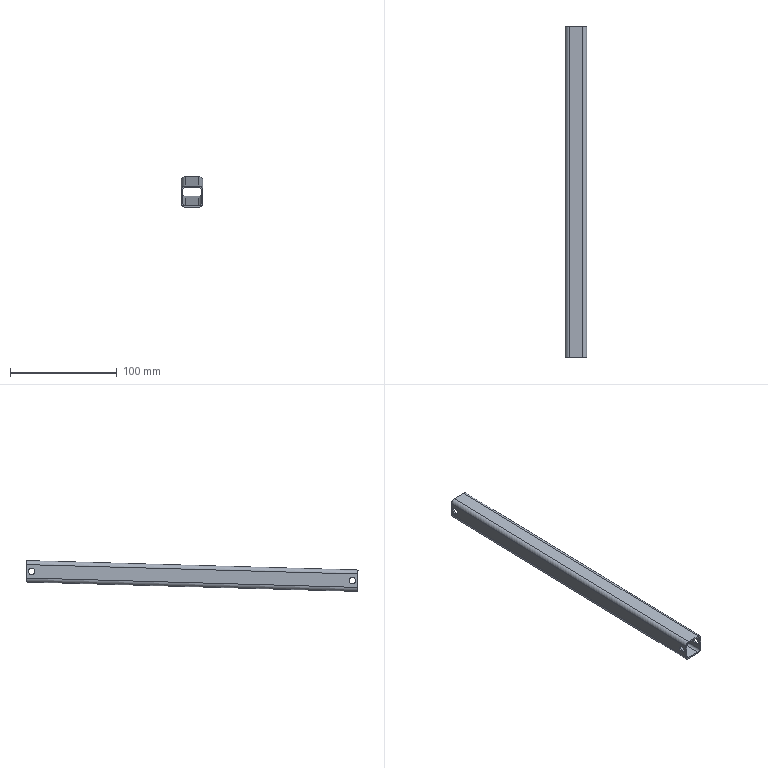Part | SolidWorks | features BaseBody 1 | 1 solid | 26 faces | box 20 x 310.443 x 28.789 mm | volume 31845 mm3 | cylinder 16 | plane 10 | commonest cylinder face diameters 6 x8 4.5 x4 7.5 x4
STEP:
#1=CARTESIAN_POINT('',(-3.273,-26.055,-774.101));
#2=VERTEX_POINT('',#1);
#3=CARTESIAN_POINT('',(-3.273,-32.052,-774.271));
#4=VERTEX_POINT('',#3);
#5=CARTESIAN_POINT('',(-3.273,-29.054,-774.186));
#6=DIRECTION('',(1.,0.,0.));
#7=DIRECTION('',(0.,-0.9996,-0.02838));
#8=AXIS2_PLACEMENT_3D('',#5,#6,#7);
#9=CIRCLE('',#8,3.);
#10=EDGE_CURVE('',#2,#4,#9,.T.);
#11=ORIENTED_EDGE('',*,*,#10,.F.);
#12=CARTESIAN_POINT('',(-1.773,-26.055,-774.101));
#13=VERTEX_POINT('',#12);
#14=CARTESIAN_POINT('',(-21.773,-26.055,-774.101));
#15=DIRECTION('',(1.,0.,0.));
#16=VECTOR('',#15,1000.);
#17=LINE('',#14,#16);
#18=EDGE_CURVE('',#2,#13,#17,.T.);
#19=ORIENTED_EDGE('',*,*,#18,.T.);
#20=CARTESIAN_POINT('',(-1.773,-32.052,-774.271));
#21=VERTEX_POINT('',#20);
#22=CARTESIAN_POINT('',(-1.773,-29.054,-774.186));
#23=DIRECTION('',(-1.,0.,0.));
#24=DIRECTION('',(0.,-0.9996,-0.02838));
#25=AXIS2_PLACEMENT_3D('',#22,#23,#24);
#26=CIRCLE('',#25,3.);
#27=EDGE_CURVE('',#21,#13,#26,.T.);
#28=ORIENTED_EDGE('',*,*,#27,.F.);
#29=CARTESIAN_POINT('',(-21.773,-32.052,-774.271));
#30=DIRECTION('',(1.,0.,0.));
#31=VECTOR('',#30,1000.);
#32=LINE('',#29,#31);
#33=EDGE_CURVE('',#4,#21,#32,.T.);
#34=ORIENTED_EDGE('',*,*,#33,.F.);
#35=EDGE_LOOP('',(#11,#19,#28,#34));
#36=FACE_OUTER_BOUND('',#35,.T.);
#37=CARTESIAN_POINT('',(-21.773,-29.054,-774.186));
#38=DIRECTION('',(1.,0.,0.));
#39=DIRECTION('',(0.,-0.9996,-0.02838));
#40=AXIS2_PLACEMENT_3D('',#37,#38,#39);
#41=CYLINDRICAL_SURFACE('',#40,3.);
#42=ADVANCED_FACE('',(#36),#41,.F.);
#43=CARTESIAN_POINT('',(-21.773,-26.055,-774.101));
#44=VERTEX_POINT('',#43);
#45=CARTESIAN_POINT('',(-21.773,-32.052,-774.271));
#46=VERTEX_POINT('',#45);
#47=CARTESIAN_POINT('',(-21.773,-29.054,-774.186));
#48=DIRECTION('',(1.,0.,0.));
#49=DIRECTION('',(0.,-0.9996,-0.02838));
#50=AXIS2_PLACEMENT_3D('',#47,#48,#49);
#51=CIRCLE('',#50,3.);
#52=EDGE_CURVE('',#44,#46,#51,.T.);
#53=ORIENTED_EDGE('',*,*,#52,.F.);
#54=CARTESIAN_POINT('',(-20.273,-26.055,-774.101));
#55=VERTEX_POINT('',#54);
#56=CARTESIAN_POINT('',(-21.773,-26.055,-774.101));
#57=DIRECTION('',(1.,0.,0.));
#58=VECTOR('',#57,1000.);
#59=LINE('',#56,#58);
#60=EDGE_CURVE('',#44,#55,#59,.T.);
#61=ORIENTED_EDGE('',*,*,#60,.T.);
#62=CARTESIAN_POINT('',(-20.273,-32.052,-774.271));
#63=VERTEX_POINT('',#62);
#64=CARTESIAN_POINT('',(-20.273,-29.054,-774.186));
#65=DIRECTION('',(-1.,0.,0.));
#66=DIRECTION('',(0.,-0.9996,-0.02838));
#67=AXIS2_PLACEMENT_3D('',#64,#65,#66);
#68=CIRCLE('',#67,3.);
#69=EDGE_CURVE('',#63,#55,#68,.T.);
#70=ORIENTED_EDGE('',*,*,#69,.F.);
#71=CARTESIAN_POINT('',(-21.773,-32.052,-774.271));
#72=DIRECTION('',(1.,0.,0.));
#73=VECTOR('',#72,1000.);
#74=LINE('',#71,#73);
#75=EDGE_CURVE('',#46,#63,#74,.T.);
#76=ORIENTED_EDGE('',*,*,#75,.F.);
#77=EDGE_LOOP('',(#53,#61,#70,#76));
#78=FACE_OUTER_BOUND('',#77,.T.);
#79=CARTESIAN_POINT('',(-21.773,-29.054,-774.186));
#80=DIRECTION('',(1.,0.,0.));
#81=DIRECTION('',(0.,-0.9996,-0.02838));
#82=AXIS2_PLACEMENT_3D('',#79,#80,#81);
#83=CYLINDRICAL_SURFACE('',#82,3.);
#84=ADVANCED_FACE('',(#78),#83,.F.);
#85=CARTESIAN_POINT('',(-3.273,273.824,-765.587));
#86=VERTEX_POINT('',#85);
#87=CARTESIAN_POINT('',(-3.273,267.827,-765.757));
#88=VERTEX_POINT('',#87);
#89=CARTESIAN_POINT('',(-3.273,270.826,-765.672));
#90=DIRECTION('',(1.,0.,0.));
#91=DIRECTION('',(0.,-0.9996,-0.02838));
#92=AXIS2_PLACEMENT_3D('',#89,#90,#91);
#93=CIRCLE('',#92,3.);
#94=EDGE_CURVE('',#86,#88,#93,.T.);
#95=ORIENTED_EDGE('',*,*,#94,.F.);
#96=CARTESIAN_POINT('',(-1.773,273.824,-765.587));
#97=VERTEX_POINT('',#96);
#98=CARTESIAN_POINT('',(-21.773,273.824,-765.587));
#99=DIRECTION('',(1.,0.,0.));
#100=VECTOR('',#99,1000.);
#101=LINE('',#98,#100);
#102=EDGE_CURVE('',#86,#97,#101,.T.);
#103=ORIENTED_EDGE('',*,*,#102,.T.);
#104=CARTESIAN_POINT('',(-1.773,267.827,-765.757));
#105=VERTEX_POINT('',#104);
#106=CARTESIAN_POINT('',(-1.773,270.826,-765.672));
#107=DIRECTION('',(-1.,0.,0.));
#108=DIRECTION('',(0.,-0.9996,-0.02838));
#109=AXIS2_PLACEMENT_3D('',#106,#107,#108);
#110=CIRCLE('',#109,3.);
#111=EDGE_CURVE('',#105,#97,#110,.T.);
#112=ORIENTED_EDGE('',*,*,#111,.F.);
#113=CARTESIAN_POINT('',(-21.773,267.827,-765.757));
#114=DIRECTION('',(1.,0.,0.));
#115=VECTOR('',#114,1000.);
#116=LINE('',#113,#115);
#117=EDGE_CURVE('',#88,#105,#116,.T.);
#118=ORIENTED_EDGE('',*,*,#117,.F.);
#119=EDGE_LOOP('',(#95,#103,#112,#118));
#120=FACE_OUTER_BOUND('',#119,.T.);
#121=CARTESIAN_POINT('',(-21.773,270.826,-765.672));
#122=DIRECTION('',(1.,0.,0.));
#123=DIRECTION('',(0.,-0.9996,-0.02838));
#124=AXIS2_PLACEMENT_3D('',#121,#122,#123);
#125=CYLINDRICAL_SURFACE('',#124,3.);
#126=ADVANCED_FACE('',(#120),#125,.F.);
#127=CARTESIAN_POINT('',(-21.773,273.824,-765.587));
#128=VERTEX_POINT('',#127);
#129=CARTESIAN_POINT('',(-21.773,267.827,-765.757));
#130=VERTEX_POINT('',#129);
#131=CARTESIAN_POINT('',(-21.773,270.826,-765.672));
#132=DIRECTION('',(1.,0.,0.));
#133=DIRECTION('',(0.,-0.9996,-0.02838));
#134=AXIS2_PLACEMENT_3D('',#131,#132,#133);
#135=CIRCLE('',#134,3.);
#136=EDGE_CURVE('',#128,#130,#135,.T.);
#137=ORIENTED_EDGE('',*,*,#136,.F.);
#138=CARTESIAN_POINT('',(-20.273,273.824,-765.587));
#139=VERTEX_POINT('',#138);
#140=CARTESIAN_POINT('',(-21.773,273.824,-765.587));
#141=DIRECTION('',(1.,0.,0.));
#142=VECTOR('',#141,1000.);
#143=LINE('',#140,#142);
#144=EDGE_CURVE('',#128,#139,#143,.T.);
#145=ORIENTED_EDGE('',*,*,#144,.T.);
#146=CARTESIAN_POINT('',(-20.273,267.827,-765.757));
#147=VERTEX_POINT('',#146);
#148=CARTESIAN_POINT('',(-20.273,270.826,-765.672));
#149=DIRECTION('',(-1.,0.,0.));
#150=DIRECTION('',(0.,-0.9996,-0.02838));
#151=AXIS2_PLACEMENT_3D('',#148,#149,#150);
#152=CIRCLE('',#151,3.);
#153=EDGE_CURVE('',#147,#139,#152,.T.);
#154=ORIENTED_EDGE('',*,*,#153,.F.);
#155=CARTESIAN_POINT('',(-21.773,267.827,-765.757));
#156=DIRECTION('',(1.,0.,0.));
#157=VECTOR('',#156,1000.);
#158=LINE('',#155,#157);
#159=EDGE_CURVE('',#130,#147,#158,.T.);
#160=ORIENTED_EDGE('',*,*,#159,.F.);
#161=EDGE_LOOP('',(#137,#145,#154,#160));
#162=FACE_OUTER_BOUND('',#161,.T.);
#163=CARTESIAN_POINT('',(-21.773,270.826,-765.672));
#164=DIRECTION('',(1.,0.,0.));
#165=DIRECTION('',(0.,-0.9996,-0.02838));
#166=AXIS2_PLACEMENT_3D('',#163,#164,#165);
#167=CYLINDRICAL_SURFACE('',#166,3.);
#168=ADVANCED_FACE('',(#162),#167,.F.);
#169=CARTESIAN_POINT('',(-18.023,-33.81,-782.824));
#170=VERTEX_POINT('',#169);
#171=CARTESIAN_POINT('',(-5.523,-33.81,-782.824));
#172=VERTEX_POINT('',#171);
#173=CARTESIAN_POINT('',(-8.648,-33.81,-782.824));
#174=DIRECTION('',(1.,0.,0.));
#175=VECTOR('',#174,1000.);
#176=LINE('',#173,#175);
#177=EDGE_CURVE('',#170,#172,#176,.T.);
#178=ORIENTED_EDGE('',*,*,#177,.F.);
#179=CARTESIAN_POINT('',(-20.273,-33.874,-780.575));
#180=VERTEX_POINT('',#179);
#181=CARTESIAN_POINT('',(-18.023,-33.874,-780.575));
#182=DIRECTION('',(0.,-0.9996,-0.02838));
#183=DIRECTION('',(1.,0.,0.));
#184=AXIS2_PLACEMENT_3D('',#181,#182,#183);
#185=CIRCLE('',#184,2.25);
#186=EDGE_CURVE('',#180,#170,#185,.T.);
#187=ORIENTED_EDGE('',*,*,#186,.F.);
#188=CARTESIAN_POINT('',(-20.273,-34.229,-768.08));
#189=VERTEX_POINT('',#188);
#190=CARTESIAN_POINT('',(-20.273,-33.963,-777.451));
#191=DIRECTION('',(0.,0.02838,-0.9996));
#192=VECTOR('',#191,1000.);
#193=LINE('',#190,#192);
#194=EDGE_CURVE('',#189,#180,#193,.T.);
#195=ORIENTED_EDGE('',*,*,#194,.F.);
#196=CARTESIAN_POINT('',(-18.023,-34.293,-765.831));
#197=VERTEX_POINT('',#196);
#198=CARTESIAN_POINT('',(-18.023,-34.229,-768.08));
#199=DIRECTION('',(0.,-0.9996,-0.02838));
#200=DIRECTION('',(0.,0.02838,-0.9996));
#201=AXIS2_PLACEMENT_3D('',#198,#199,#200);
#202=CIRCLE('',#201,2.25);
#203=EDGE_CURVE('',#197,#189,#202,.T.);
#204=ORIENTED_EDGE('',*,*,#203,.F.);
#205=CARTESIAN_POINT('',(-5.523,-34.293,-765.831));
#206=VERTEX_POINT('',#205);
#207=CARTESIAN_POINT('',(-14.898,-34.293,-765.831));
#208=DIRECTION('',(-1.,0.,0.));
#209=VECTOR('',#208,1000.);
#210=LINE('',#207,#209);
#211=EDGE_CURVE('',#206,#197,#210,.T.);
#212=ORIENTED_EDGE('',*,*,#211,.F.);
#213=CARTESIAN_POINT('',(-3.273,-34.229,-768.08));
#214=VERTEX_POINT('',#213);
#215=CARTESIAN_POINT('',(-5.523,-34.229,-768.08));
#216=DIRECTION('',(0.,-0.9996,-0.02838));
#217=DIRECTION('',(-1.,0.,0.));
#218=AXIS2_PLACEMENT_3D('',#215,#216,#217);
#219=CIRCLE('',#218,2.25);
#220=EDGE_CURVE('',#214,#206,#219,.T.);
#221=ORIENTED_EDGE('',*,*,#220,.F.);
#222=CARTESIAN_POINT('',(-3.273,-33.874,-780.575));
#223=VERTEX_POINT('',#222);
#224=CARTESIAN_POINT('',(-3.273,-34.14,-771.204));
#225=DIRECTION('',(0.,-0.02838,0.9996));
#226=VECTOR('',#225,1000.);
#227=LINE('',#224,#226);
#228=EDGE_CURVE('',#223,#214,#227,.T.);
#229=ORIENTED_EDGE('',*,*,#228,.F.);
#230=CARTESIAN_POINT('',(-5.523,-33.874,-780.575));
#231=DIRECTION('',(0.,-0.9996,-0.02838));
#232=DIRECTION('',(0.,-0.02838,0.9996));
#233=AXIS2_PLACEMENT_3D('',#230,#231,#232);
#234=CIRCLE('',#233,2.25);
#235=EDGE_CURVE('',#172,#223,#234,.T.);
#236=ORIENTED_EDGE('',*,*,#235,.F.);
#237=EDGE_LOOP('',(#178,#187,#195,#204,#212,#221,#229,#236));
#238=FACE_BOUND('',#237,.T.);
#239=CARTESIAN_POINT('',(-1.773,-34.229,-768.08));
#240=VERTEX_POINT('',#239);
#241=CARTESIAN_POINT('',(-1.773,-33.874,-780.575));
#242=VERTEX_POINT('',#241);
#243=CARTESIAN_POINT('',(-1.773,-34.14,-771.204));
#244=DIRECTION('',(0.,0.02838,-0.9996));
#245=VECTOR('',#244,1000.);
#246=LINE('',#243,#245);
#247=EDGE_CURVE('',#240,#242,#246,.T.);
#248=ORIENTED_EDGE('',*,*,#247,.F.);
#249=CARTESIAN_POINT('',(-5.523,-34.335,-764.332));
#250=VERTEX_POINT('',#249);
#251=CARTESIAN_POINT('',(-5.523,-34.229,-768.08));
#252=DIRECTION('',(0.,0.9996,0.02838));
#253=DIRECTION('',(-1.,0.,0.));
#254=AXIS2_PLACEMENT_3D('',#251,#252,#253);
#255=CIRCLE('',#254,3.75);
#256=EDGE_CURVE('',#250,#240,#255,.T.);
#257=ORIENTED_EDGE('',*,*,#256,.F.);
#258=CARTESIAN_POINT('',(-18.023,-34.335,-764.332));
#259=VERTEX_POINT('',#258);
#260=CARTESIAN_POINT('',(-14.898,-34.335,-764.332));
#261=DIRECTION('',(1.,0.,0.));
#262=VECTOR('',#261,1000.);
#263=LINE('',#260,#262);
#264=EDGE_CURVE('',#259,#250,#263,.T.);
#265=ORIENTED_EDGE('',*,*,#264,.F.);
#266=CARTESIAN_POINT('',(-21.773,-34.229,-768.08));
#267=VERTEX_POINT('',#266);
#268=CARTESIAN_POINT('',(-18.023,-34.229,-768.08));
#269=DIRECTION('',(0.,0.9996,0.02838));
#270=DIRECTION('',(0.,0.02838,-0.9996));
#271=AXIS2_PLACEMENT_3D('',#268,#269,#270);
#272=CIRCLE('',#271,3.75);
#273=EDGE_CURVE('',#267,#259,#272,.T.);
#274=ORIENTED_EDGE('',*,*,#273,.F.);
#275=CARTESIAN_POINT('',(-21.773,-33.874,-780.575));
#276=VERTEX_POINT('',#275);
#277=CARTESIAN_POINT('',(-21.773,-33.963,-777.451));
#278=DIRECTION('',(0.,-0.02838,0.9996));
#279=VECTOR('',#278,1000.);
#280=LINE('',#277,#279);
#281=EDGE_CURVE('',#276,#267,#280,.T.);
#282=ORIENTED_EDGE('',*,*,#281,.F.);
#283=CARTESIAN_POINT('',(-18.023,-33.768,-784.324));
#284=VERTEX_POINT('',#283);
#285=CARTESIAN_POINT('',(-18.023,-33.874,-780.575));
#286=DIRECTION('',(0.,0.9996,0.02838));
#287=DIRECTION('',(1.,0.,0.));
#288=AXIS2_PLACEMENT_3D('',#285,#286,#287);
#289=CIRCLE('',#288,3.75);
#290=EDGE_CURVE('',#284,#276,#289,.T.);
#291=ORIENTED_EDGE('',*,*,#290,.F.);
#292=CARTESIAN_POINT('',(-5.523,-33.768,-784.324));
#293=VERTEX_POINT('',#292);
#294=CARTESIAN_POINT('',(-8.648,-33.768,-784.324));
#295=DIRECTION('',(-1.,0.,0.));
#296=VECTOR('',#295,1000.);
#297=LINE('',#294,#296);
#298=EDGE_CURVE('',#293,#284,#297,.T.);
#299=ORIENTED_EDGE('',*,*,#298,.F.);
#300=CARTESIAN_POINT('',(-5.523,-33.874,-780.575));
#301=DIRECTION('',(0.,0.9996,0.02838));
#302=DIRECTION('',(0.,-0.02838,0.9996));
#303=AXIS2_PLACEMENT_3D('',#300,#301,#302);
#304=CIRCLE('',#303,3.75);
#305=EDGE_CURVE('',#242,#293,#304,.T.);
#306=ORIENTED_EDGE('',*,*,#305,.F.);
#307=EDGE_LOOP('',(#248,#257,#265,#274,#282,#291,#299,#306));
#308=FACE_OUTER_BOUND('',#307,.T.);
#309=CARTESIAN_POINT('',(-11.773,-34.052,-774.328));
#310=DIRECTION('',(0.,-0.9996,-0.02838));
#311=DIRECTION('',(-1.,0.,0.));
#312=AXIS2_PLACEMENT_3D('',#309,#310,#311);
#313=PLANE('',#312);
#314=ADVANCED_FACE('',(#238,#308),#313,.T.);
#315=CARTESIAN_POINT('',(-18.023,276.065,-774.027));
#316=VERTEX_POINT('',#315);
#317=CARTESIAN_POINT('',(-5.523,276.065,-774.027));
#318=VERTEX_POINT('',#317);
#319=CARTESIAN_POINT('',(-8.648,276.065,-774.027));
#320=DIRECTION('',(1.,0.,0.));
#321=VECTOR('',#320,1000.);
#322=LINE('',#319,#321);
#323=EDGE_CURVE('',#316,#318,#322,.T.);
#324=ORIENTED_EDGE('',*,*,#323,.T.);
#325=CARTESIAN_POINT('',(-3.273,276.001,-771.778));
#326=VERTEX_POINT('',#325);
#327=CARTESIAN_POINT('',(-5.523,276.001,-771.778));
#328=DIRECTION('',(0.,-0.9996,-0.02838));
#329=DIRECTION('',(0.,-0.02838,0.9996));
#330=AXIS2_PLACEMENT_3D('',#327,#328,#329);
#331=CIRCLE('',#330,2.25);
#332=EDGE_CURVE('',#318,#326,#331,.T.);
#333=ORIENTED_EDGE('',*,*,#332,.T.);
#334=CARTESIAN_POINT('',(-3.273,275.646,-759.283));
#335=VERTEX_POINT('',#334);
#336=CARTESIAN_POINT('',(-3.273,275.735,-762.406));
#337=DIRECTION('',(0.,-0.02838,0.9996));
#338=VECTOR('',#337,1000.);
#339=LINE('',#336,#338);
#340=EDGE_CURVE('',#326,#335,#339,.T.);
#341=ORIENTED_EDGE('',*,*,#340,.T.);
#342=CARTESIAN_POINT('',(-5.523,275.582,-757.034));
#343=VERTEX_POINT('',#342);
#344=CARTESIAN_POINT('',(-5.523,275.646,-759.283));
#345=DIRECTION('',(0.,-0.9996,-0.02838));
#346=DIRECTION('',(-1.,0.,0.));
#347=AXIS2_PLACEMENT_3D('',#344,#345,#346);
#348=CIRCLE('',#347,2.25);
#349=EDGE_CURVE('',#335,#343,#348,.T.);
#350=ORIENTED_EDGE('',*,*,#349,.T.);
#351=CARTESIAN_POINT('',(-18.023,275.582,-757.034));
#352=VERTEX_POINT('',#351);
#353=CARTESIAN_POINT('',(-14.898,275.582,-757.034));
#354=DIRECTION('',(-1.,0.,0.));
#355=VECTOR('',#354,1000.);
#356=LINE('',#353,#355);
#357=EDGE_CURVE('',#343,#352,#356,.T.);
#358=ORIENTED_EDGE('',*,*,#357,.T.);
#359=CARTESIAN_POINT('',(-20.273,275.646,-759.283));
#360=VERTEX_POINT('',#359);
#361=CARTESIAN_POINT('',(-18.023,275.646,-759.283));
#362=DIRECTION('',(0.,-0.9996,-0.02838));
#363=DIRECTION('',(0.,0.02838,-0.9996));
#364=AXIS2_PLACEMENT_3D('',#361,#362,#363);
#365=CIRCLE('',#364,2.25);
#366=EDGE_CURVE('',#352,#360,#365,.T.);
#367=ORIENTED_EDGE('',*,*,#366,.T.);
#368=CARTESIAN_POINT('',(-20.273,276.001,-771.778));
#369=VERTEX_POINT('',#368);
#370=CARTESIAN_POINT('',(-20.273,275.912,-768.654));
#371=DIRECTION('',(0.,0.02838,-0.9996));
#372=VECTOR('',#371,1000.);
#373=LINE('',#370,#372);
#374=EDGE_CURVE('',#360,#369,#373,.T.);
#375=ORIENTED_EDGE('',*,*,#374,.T.);
#376=CARTESIAN_POINT('',(-18.023,276.001,-771.778));
#377=DIRECTION('',(0.,-0.9996,-0.02838));
#378=DIRECTION('',(1.,0.,0.));
#379=AXIS2_PLACEMENT_3D('',#376,#377,#378);
#380=CIRCLE('',#379,2.25);
#381=EDGE_CURVE('',#369,#316,#380,.T.);
#382=ORIENTED_EDGE('',*,*,#381,.T.);
#383=EDGE_LOOP('',(#324,#333,#341,#350,#358,#367,#375,#382));
#384=FACE_BOUND('',#383,.T.);
#385=CARTESIAN_POINT('',(-1.773,275.646,-759.283));
#386=VERTEX_POINT('',#385);
#387=CARTESIAN_POINT('',(-1.773,276.001,-771.778));
#388=VERTEX_POINT('',#387);
#389=CARTESIAN_POINT('',(-1.773,275.735,-762.406));
#390=DIRECTION('',(0.,0.02838,-0.9996));
#391=VECTOR('',#390,1000.);
#392=LINE('',#389,#391);
#393=EDGE_CURVE('',#386,#388,#392,.T.);
#394=ORIENTED_EDGE('',*,*,#393,.T.);
#395=CARTESIAN_POINT('',(-5.523,276.107,-775.526));
#396=VERTEX_POINT('',#395);
#397=CARTESIAN_POINT('',(-5.523,276.001,-771.778));
#398=DIRECTION('',(0.,0.9996,0.02838));
#399=DIRECTION('',(0.,-0.02838,0.9996));
#400=AXIS2_PLACEMENT_3D('',#397,#398,#399);
#401=CIRCLE('',#400,3.75);
#402=EDGE_CURVE('',#388,#396,#401,.T.);
#403=ORIENTED_EDGE('',*,*,#402,.T.);
#404=CARTESIAN_POINT('',(-18.023,276.107,-775.526));
#405=VERTEX_POINT('',#404);
#406=CARTESIAN_POINT('',(-8.648,276.107,-775.526));
#407=DIRECTION('',(-1.,0.,0.));
#408=VECTOR('',#407,1000.);
#409=LINE('',#406,#408);
#410=EDGE_CURVE('',#396,#405,#409,.T.);
#411=ORIENTED_EDGE('',*,*,#410,.T.);
#412=CARTESIAN_POINT('',(-21.773,276.001,-771.778));
#413=VERTEX_POINT('',#412);
#414=CARTESIAN_POINT('',(-18.023,276.001,-771.778));
#415=DIRECTION('',(0.,0.9996,0.02838));
#416=DIRECTION('',(1.,0.,0.));
#417=AXIS2_PLACEMENT_3D('',#414,#415,#416);
#418=CIRCLE('',#417,3.75);
#419=EDGE_CURVE('',#405,#413,#418,.T.);
#420=ORIENTED_EDGE('',*,*,#419,.T.);
#421=CARTESIAN_POINT('',(-21.773,275.646,-759.283));
#422=VERTEX_POINT('',#421);
#423=CARTESIAN_POINT('',(-21.773,275.912,-768.654));
#424=DIRECTION('',(0.,-0.02838,0.9996));
#425=VECTOR('',#424,1000.);
#426=LINE('',#423,#425);
#427=EDGE_CURVE('',#413,#422,#426,.T.);
#428=ORIENTED_EDGE('',*,*,#427,.T.);
#429=CARTESIAN_POINT('',(-18.023,275.54,-755.534));
#430=VERTEX_POINT('',#429);
#431=CARTESIAN_POINT('',(-18.023,275.646,-759.283));
#432=DIRECTION('',(0.,0.9996,0.02838));
#433=DIRECTION('',(0.,0.02838,-0.9996));
#434=AXIS2_PLACEMENT_3D('',#431,#432,#433);
#435=CIRCLE('',#434,3.75);
#436=EDGE_CURVE('',#422,#430,#435,.T.);
#437=ORIENTED_EDGE('',*,*,#436,.T.);
#438=CARTESIAN_POINT('',(-5.523,275.54,-755.534));
#439=VERTEX_POINT('',#438);
#440=CARTESIAN_POINT('',(-14.898,275.54,-755.534));
#441=DIRECTION('',(1.,0.,0.));
#442=VECTOR('',#441,1000.);
#443=LINE('',#440,#442);
#444=EDGE_CURVE('',#430,#439,#443,.T.);
#445=ORIENTED_EDGE('',*,*,#444,.T.);
#446=CARTESIAN_POINT('',(-5.523,275.646,-759.283));
#447=DIRECTION('',(0.,0.9996,0.02838));
#448=DIRECTION('',(-1.,0.,0.));
#449=AXIS2_PLACEMENT_3D('',#446,#447,#448);
#450=CIRCLE('',#449,3.75);
#451=EDGE_CURVE('',#439,#386,#450,.T.);
#452=ORIENTED_EDGE('',*,*,#451,.T.);
#453=EDGE_LOOP('',(#394,#403,#411,#420,#428,#437,#445,#452));
#454=FACE_OUTER_BOUND('',#453,.T.);
#455=CARTESIAN_POINT('',(-11.773,275.823,-765.53));
#456=DIRECTION('',(0.,-0.9996,-0.02838));
#457=DIRECTION('',(-1.,0.,0.));
#458=AXIS2_PLACEMENT_3D('',#455,#456,#457);
#459=PLANE('',#458);
#460=ADVANCED_FACE('',(#384,#454),#459,.F.);
#461=ORIENTED_EDGE('',*,*,#290,.T.);
#462=CARTESIAN_POINT('',(-21.773,276.001,-771.778));
#463=DIRECTION('',(0.,-0.9996,-0.02838));
#464=VECTOR('',#463,1000.);
#465=LINE('',#462,#464);
#466=EDGE_CURVE('',#413,#276,#465,.T.);
#467=ORIENTED_EDGE('',*,*,#466,.F.);
#468=ORIENTED_EDGE('',*,*,#419,.F.);
#469=CARTESIAN_POINT('',(-18.023,276.107,-775.526));
#470=DIRECTION('',(0.,-0.9996,-0.02838));
#471=VECTOR('',#470,1000.);
#472=LINE('',#469,#471);
#473=EDGE_CURVE('',#405,#284,#472,.T.);
#474=ORIENTED_EDGE('',*,*,#473,.T.);
#475=EDGE_LOOP('',(#461,#467,#468,#474));
#476=FACE_OUTER_BOUND('',#475,.T.);
#477=CARTESIAN_POINT('',(-18.023,276.001,-771.778));
#478=DIRECTION('',(0.,-0.9996,-0.02838));
#479=DIRECTION('',(1.,0.,0.));
#480=AXIS2_PLACEMENT_3D('',#477,#478,#479);
#481=CYLINDRICAL_SURFACE('',#480,3.75);
#482=ADVANCED_FACE('',(#476),#481,.T.);
#483=ORIENTED_EDGE('',*,*,#298,.T.);
#484=ORIENTED_EDGE('',*,*,#473,.F.);
#485=ORIENTED_EDGE('',*,*,#410,.F.);
#486=CARTESIAN_POINT('',(-5.523,276.107,-775.526));
#487=DIRECTION('',(0.,-0.9996,-0.02838));
#488=VECTOR('',#487,1000.);
#489=LINE('',#486,#488);
#490=EDGE_CURVE('',#396,#293,#489,.T.);
#491=ORIENTED_EDGE('',*,*,#490,.T.);
#492=EDGE_LOOP('',(#483,#484,#485,#491));
#493=FACE_OUTER_BOUND('',#492,.T.);
#494=CARTESIAN_POINT('',(-5.523,276.107,-775.526));
#495=DIRECTION('',(0.,0.02838,-0.9996));
#496=DIRECTION('',(-1.,0.,0.));
#497=AXIS2_PLACEMENT_3D('',#494,#495,#496);
#498=PLANE('',#497);
#499=ADVANCED_FACE('',(#493),#498,.T.);
#500=ORIENTED_EDGE('',*,*,#305,.T.);
#501=ORIENTED_EDGE('',*,*,#490,.F.);
#502=ORIENTED_EDGE('',*,*,#402,.F.);
#503=CARTESIAN_POINT('',(-1.773,276.001,-771.778));
#504=DIRECTION('',(0.,-0.9996,-0.02838));
#505=VECTOR('',#504,1000.);
#506=LINE('',#503,#505);
#507=EDGE_CURVE('',#388,#242,#506,.T.);
#508=ORIENTED_EDGE('',*,*,#507,.T.);
#509=EDGE_LOOP('',(#500,#501,#502,#508));
#510=FACE_OUTER_BOUND('',#509,.T.);
#511=CARTESIAN_POINT('',(-5.523,276.001,-771.778));
#512=DIRECTION('',(0.,-0.9996,-0.02838));
#513=DIRECTION('',(0.,-0.02838,0.9996));
#514=AXIS2_PLACEMENT_3D('',#511,#512,#513);
#515=CYLINDRICAL_SURFACE('',#514,3.75);
#516=ADVANCED_FACE('',(#510),#515,.T.);
#517=ORIENTED_EDGE('',*,*,#111,.T.);
#518=CARTESIAN_POINT('',(-1.773,270.826,-765.672));
#519=DIRECTION('',(-1.,0.,0.));
#520=DIRECTION('',(0.,-0.9996,-0.02838));
#521=AXIS2_PLACEMENT_3D('',#518,#519,#520);
#522=CIRCLE('',#521,3.);
#523=EDGE_CURVE('',#97,#105,#522,.T.);
#524=ORIENTED_EDGE('',*,*,#523,.T.);
#525=EDGE_LOOP('',(#517,#524));
#526=FACE_BOUND('',#525,.T.);
#527=ORIENTED_EDGE('',*,*,#27,.T.);
#528=CARTESIAN_POINT('',(-1.773,-29.054,-774.186));
#529=DIRECTION('',(-1.,0.,0.));
#530=DIRECTION('',(0.,-0.9996,-0.02838));
#531=AXIS2_PLACEMENT_3D('',#528,#529,#530);
#532=CIRCLE('',#531,3.);
#533=EDGE_CURVE('',#13,#21,#532,.T.);
#534=ORIENTED_EDGE('',*,*,#533,.T.);
#535=EDGE_LOOP('',(#527,#534));
#536=FACE_BOUND('',#535,.T.);
#537=ORIENTED_EDGE('',*,*,#247,.T.);
#538=ORIENTED_EDGE('',*,*,#507,.F.);
#539=ORIENTED_EDGE('',*,*,#393,.F.);
#540=CARTESIAN_POINT('',(-1.773,275.646,-759.283));
#541=DIRECTION('',(0.,-0.9996,-0.02838));
#542=VECTOR('',#541,1000.);
#543=LINE('',#540,#542);
#544=EDGE_CURVE('',#386,#240,#543,.T.);
#545=ORIENTED_EDGE('',*,*,#544,.T.);
#546=EDGE_LOOP('',(#537,#538,#539,#545));
#547=FACE_OUTER_BOUND('',#546,.T.);
#548=CARTESIAN_POINT('',(-1.773,275.646,-759.283));
#549=DIRECTION('',(1.,0.,0.));
#550=DIRECTION('',(0.,-0.9996,-0.02838));
#551=AXIS2_PLACEMENT_3D('',#548,#549,#550);
#552=PLANE('',#551);
#553=ADVANCED_FACE('',(#526,#536,#547),#552,.T.);
#554=ORIENTED_EDGE('',*,*,#235,.T.);
#555=CARTESIAN_POINT('',(-3.273,276.001,-771.778));
#556=DIRECTION('',(0.,-0.9996,-0.02838));
#557=VECTOR('',#556,1000.);
#558=LINE('',#555,#557);
#559=EDGE_CURVE('',#326,#223,#558,.T.);
#560=ORIENTED_EDGE('',*,*,#559,.F.);
#561=ORIENTED_EDGE('',*,*,#332,.F.);
#562=CARTESIAN_POINT('',(-5.523,276.065,-774.027));
#563=DIRECTION('',(0.,-0.9996,-0.02838));
#564=VECTOR('',#563,1000.);
#565=LINE('',#562,#564);
#566=EDGE_CURVE('',#318,#172,#565,.T.);
#567=ORIENTED_EDGE('',*,*,#566,.T.);
#568=EDGE_LOOP('',(#554,#560,#561,#567));
#569=FACE_OUTER_BOUND('',#568,.T.);
#570=CARTESIAN_POINT('',(-5.523,276.001,-771.778));
#571=DIRECTION('',(0.,-0.9996,-0.02838));
#572=DIRECTION('',(0.,-0.02838,0.9996));
#573=AXIS2_PLACEMENT_3D('',#570,#571,#572);
#574=CYLINDRICAL_SURFACE('',#573,2.25);
#575=ADVANCED_FACE('',(#569),#574,.F.);
#576=CARTESIAN_POINT('',(-3.273,270.826,-765.672));
#577=DIRECTION('',(1.,0.,0.));
#578=DIRECTION('',(0.,-0.9996,-0.02838));
#579=AXIS2_PLACEMENT_3D('',#576,#577,#578);
#580=CIRCLE('',#579,3.);
#581=EDGE_CURVE('',#88,#86,#580,.T.);
#582=ORIENTED_EDGE('',*,*,#581,.T.);
#583=ORIENTED_EDGE('',*,*,#94,.T.);
#584=EDGE_LOOP('',(#582,#583));
#585=FACE_BOUND('',#584,.T.);
#586=CARTESIAN_POINT('',(-3.273,-29.054,-774.186));
#587=DIRECTION('',(1.,0.,0.));
#588=DIRECTION('',(0.,-0.9996,-0.02838));
#589=AXIS2_PLACEMENT_3D('',#586,#587,#588);
#590=CIRCLE('',#589,3.);
#591=EDGE_CURVE('',#4,#2,#590,.T.);
#592=ORIENTED_EDGE('',*,*,#591,.T.);
#593=ORIENTED_EDGE('',*,*,#10,.T.);
#594=EDGE_LOOP('',(#592,#593));
#595=FACE_BOUND('',#594,.T.);
#596=ORIENTED_EDGE('',*,*,#228,.T.);
#597=CARTESIAN_POINT('',(-3.273,275.646,-759.283));
#598=DIRECTION('',(0.,-0.9996,-0.02838));
#599=VECTOR('',#598,1000.);
#600=LINE('',#597,#599);
#601=EDGE_CURVE('',#335,#214,#600,.T.);
#602=ORIENTED_EDGE('',*,*,#601,.F.);
#603=ORIENTED_EDGE('',*,*,#340,.F.);
#604=ORIENTED_EDGE('',*,*,#559,.T.);
#605=EDGE_LOOP('',(#596,#602,#603,#604));
#606=FACE_OUTER_BOUND('',#605,.T.);
#607=CARTESIAN_POINT('',(-3.273,275.646,-759.283));
#608=DIRECTION('',(1.,0.,0.));
#609=DIRECTION('',(0.,-0.9996,-0.02838));
#610=AXIS2_PLACEMENT_3D('',#607,#608,#609);
#611=PLANE('',#610);
#612=ADVANCED_FACE('',(#585,#595,#606),#611,.F.);
#613=ORIENTED_EDGE('',*,*,#220,.T.);
#614=CARTESIAN_POINT('',(-5.523,275.582,-757.034));
#615=DIRECTION('',(0.,-0.9996,-0.02838));
#616=VECTOR('',#615,1000.);
#617=LINE('',#614,#616);
#618=EDGE_CURVE('',#343,#206,#617,.T.);
#619=ORIENTED_EDGE('',*,*,#618,.F.);
#620=ORIENTED_EDGE('',*,*,#349,.F.);
#621=ORIENTED_EDGE('',*,*,#601,.T.);
#622=EDGE_LOOP('',(#613,#619,#620,#621));
#623=FACE_OUTER_BOUND('',#622,.T.);
#624=CARTESIAN_POINT('',(-5.523,275.646,-759.283));
#625=DIRECTION('',(0.,-0.9996,-0.02838));
#626=DIRECTION('',(-1.,0.,0.));
#627=AXIS2_PLACEMENT_3D('',#624,#625,#626);
#628=CYLINDRICAL_SURFACE('',#627,2.25);
#629=ADVANCED_FACE('',(#623),#628,.F.);
#630=ORIENTED_EDGE('',*,*,#177,.T.);
#631=ORIENTED_EDGE('',*,*,#566,.F.);
#632=ORIENTED_EDGE('',*,*,#323,.F.);
#633=CARTESIAN_POINT('',(-18.023,276.065,-774.027));
#634=DIRECTION('',(0.,-0.9996,-0.02838));
#635=VECTOR('',#634,1000.);
#636=LINE('',#633,#635);
#637=EDGE_CURVE('',#316,#170,#636,.T.);
#638=ORIENTED_EDGE('',*,*,#637,.T.);
#639=EDGE_LOOP('',(#630,#631,#632,#638));
#640=FACE_OUTER_BOUND('',#639,.T.);
#641=CARTESIAN_POINT('',(-5.523,276.065,-774.027));
#642=DIRECTION('',(0.,0.02838,-0.9996));
#643=DIRECTION('',(-1.,0.,0.));
#644=AXIS2_PLACEMENT_3D('',#641,#642,#643);
#645=PLANE('',#644);
#646=ADVANCED_FACE('',(#640),#645,.F.);
#647=ORIENTED_EDGE('',*,*,#256,.T.);
#648=ORIENTED_EDGE('',*,*,#544,.F.);
#649=ORIENTED_EDGE('',*,*,#451,.F.);
#650=CARTESIAN_POINT('',(-5.523,275.54,-755.534));
#651=DIRECTION('',(0.,-0.9996,-0.02838));
#652=VECTOR('',#651,1000.);
#653=LINE('',#650,#652);
#654=EDGE_CURVE('',#439,#250,#653,.T.);
#655=ORIENTED_EDGE('',*,*,#654,.T.);
#656=EDGE_LOOP('',(#647,#648,#649,#655));
#657=FACE_OUTER_BOUND('',#656,.T.);
#658=CARTESIAN_POINT('',(-5.523,275.646,-759.283));
#659=DIRECTION('',(0.,-0.9996,-0.02838));
#660=DIRECTION('',(-1.,0.,0.));
#661=AXIS2_PLACEMENT_3D('',#658,#659,#660);
#662=CYLINDRICAL_SURFACE('',#661,3.75);
#663=ADVANCED_FACE('',(#657),#662,.T.);
#664=ORIENTED_EDGE('',*,*,#264,.T.);
#665=ORIENTED_EDGE('',*,*,#654,.F.);
#666=ORIENTED_EDGE('',*,*,#444,.F.);
#667=CARTESIAN_POINT('',(-18.023,275.54,-755.534));
#668=DIRECTION('',(0.,-0.9996,-0.02838));
#669=VECTOR('',#668,1000.);
#670=LINE('',#667,#669);
#671=EDGE_CURVE('',#430,#259,#670,.T.);
#672=ORIENTED_EDGE('',*,*,#671,.T.);
#673=EDGE_LOOP('',(#664,#665,#666,#672));
#674=FACE_OUTER_BOUND('',#673,.T.);
#675=CARTESIAN_POINT('',(-18.023,275.54,-755.534));
#676=DIRECTION('',(0.,-0.02838,0.9996));
#677=DIRECTION('',(0.,0.9996,0.02838));
#678=AXIS2_PLACEMENT_3D('',#675,#676,#677);
#679=PLANE('',#678);
#680=ADVANCED_FACE('',(#674),#679,.T.);
#681=ORIENTED_EDGE('',*,*,#273,.T.);
#682=ORIENTED_EDGE('',*,*,#671,.F.);
#683=ORIENTED_EDGE('',*,*,#436,.F.);
#684=CARTESIAN_POINT('',(-21.773,275.646,-759.283));
#685=DIRECTION('',(0.,-0.9996,-0.02838));
#686=VECTOR('',#685,1000.);
#687=LINE('',#684,#686);
#688=EDGE_CURVE('',#422,#267,#687,.T.);
#689=ORIENTED_EDGE('',*,*,#688,.T.);
#690=EDGE_LOOP('',(#681,#682,#683,#689));
#691=FACE_OUTER_BOUND('',#690,.T.);
#692=CARTESIAN_POINT('',(-18.023,275.646,-759.283));
#693=DIRECTION('',(0.,-0.9996,-0.02838));
#694=DIRECTION('',(0.,0.02838,-0.9996));
#695=AXIS2_PLACEMENT_3D('',#692,#693,#694);
#696=CYLINDRICAL_SURFACE('',#695,3.75);
#697=ADVANCED_FACE('',(#691),#696,.T.);
#698=CARTESIAN_POINT('',(-21.773,270.826,-765.672));
#699=DIRECTION('',(1.,0.,0.));
#700=DIRECTION('',(0.,-0.9996,-0.02838));
#701=AXIS2_PLACEMENT_3D('',#698,#699,#700);
#702=CIRCLE('',#701,3.);
#703=EDGE_CURVE('',#130,#128,#702,.T.);
#704=ORIENTED_EDGE('',*,*,#703,.T.);
#705=ORIENTED_EDGE('',*,*,#136,.T.);
#706=EDGE_LOOP('',(#704,#705));
#707=FACE_BOUND('',#706,.T.);
#708=CARTESIAN_POINT('',(-21.773,-29.054,-774.186));
#709=DIRECTION('',(1.,0.,0.));
#710=DIRECTION('',(0.,-0.9996,-0.02838));
#711=AXIS2_PLACEMENT_3D('',#708,#709,#710);
#712=CIRCLE('',#711,3.);
#713=EDGE_CURVE('',#46,#44,#712,.T.);
#714=ORIENTED_EDGE('',*,*,#713,.T.);
#715=ORIENTED_EDGE('',*,*,#52,.T.);
#716=EDGE_LOOP('',(#714,#715));
#717=FACE_BOUND('',#716,.T.);
#718=ORIENTED_EDGE('',*,*,#281,.T.);
#719=ORIENTED_EDGE('',*,*,#688,.F.);
#720=ORIENTED_EDGE('',*,*,#427,.F.);
#721=ORIENTED_EDGE('',*,*,#466,.T.);
#722=EDGE_LOOP('',(#718,#719,#720,#721));
#723=FACE_OUTER_BOUND('',#722,.T.);
#724=CARTESIAN_POINT('',(-21.773,276.001,-771.778));
#725=DIRECTION('',(-1.,0.,0.));
#726=DIRECTION('',(0.,0.02838,-0.9996));
#727=AXIS2_PLACEMENT_3D('',#724,#725,#726);
#728=PLANE('',#727);
#729=ADVANCED_FACE('',(#707,#717,#723),#728,.T.);
#730=ORIENTED_EDGE('',*,*,#186,.T.);
#731=ORIENTED_EDGE('',*,*,#637,.F.);
#732=ORIENTED_EDGE('',*,*,#381,.F.);
#733=CARTESIAN_POINT('',(-20.273,276.001,-771.778));
#734=DIRECTION('',(0.,-0.9996,-0.02838));
#735=VECTOR('',#734,1000.);
#736=LINE('',#733,#735);
#737=EDGE_CURVE('',#369,#180,#736,.T.);
#738=ORIENTED_EDGE('',*,*,#737,.T.);
#739=EDGE_LOOP('',(#730,#731,#732,#738));
#740=FACE_OUTER_BOUND('',#739,.T.);
#741=CARTESIAN_POINT('',(-18.023,276.001,-771.778));
#742=DIRECTION('',(0.,-0.9996,-0.02838));
#743=DIRECTION('',(1.,0.,0.));
#744=AXIS2_PLACEMENT_3D('',#741,#742,#743);
#745=CYLINDRICAL_SURFACE('',#744,2.25);
#746=ADVANCED_FACE('',(#740),#745,.F.);
#747=ORIENTED_EDGE('',*,*,#153,.T.);
#748=CARTESIAN_POINT('',(-20.273,270.826,-765.672));
#749=DIRECTION('',(-1.,0.,0.));
#750=DIRECTION('',(0.,-0.9996,-0.02838));
#751=AXIS2_PLACEMENT_3D('',#748,#749,#750);
#752=CIRCLE('',#751,3.);
#753=EDGE_CURVE('',#139,#147,#752,.T.);
#754=ORIENTED_EDGE('',*,*,#753,.T.);
#755=EDGE_LOOP('',(#747,#754));
#756=FACE_BOUND('',#755,.T.);
#757=ORIENTED_EDGE('',*,*,#69,.T.);
#758=CARTESIAN_POINT('',(-20.273,-29.054,-774.186));
#759=DIRECTION('',(-1.,0.,0.));
#760=DIRECTION('',(0.,-0.9996,-0.02838));
#761=AXIS2_PLACEMENT_3D('',#758,#759,#760);
#762=CIRCLE('',#761,3.);
#763=EDGE_CURVE('',#55,#63,#762,.T.);
#764=ORIENTED_EDGE('',*,*,#763,.T.);
#765=EDGE_LOOP('',(#757,#764));
#766=FACE_BOUND('',#765,.T.);
#767=ORIENTED_EDGE('',*,*,#194,.T.);
#768=ORIENTED_EDGE('',*,*,#737,.F.);
#769=ORIENTED_EDGE('',*,*,#374,.F.);
#770=CARTESIAN_POINT('',(-20.273,275.646,-759.283));
#771=DIRECTION('',(0.,-0.9996,-0.02838));
#772=VECTOR('',#771,1000.);
#773=LINE('',#770,#772);
#774=EDGE_CURVE('',#360,#189,#773,.T.);
#775=ORIENTED_EDGE('',*,*,#774,.T.);
#776=EDGE_LOOP('',(#767,#768,#769,#775));
#777=FACE_OUTER_BOUND('',#776,.T.);
#778=CARTESIAN_POINT('',(-20.273,276.001,-771.778));
#779=DIRECTION('',(-1.,0.,0.));
#780=DIRECTION('',(0.,0.02838,-0.9996));
#781=AXIS2_PLACEMENT_3D('',#778,#779,#780);
#782=PLANE('',#781);
#783=ADVANCED_FACE('',(#756,#766,#777),#782,.F.);
#784=ORIENTED_EDGE('',*,*,#203,.T.);
#785=ORIENTED_EDGE('',*,*,#774,.F.);
#786=ORIENTED_EDGE('',*,*,#366,.F.);
#787=CARTESIAN_POINT('',(-18.023,275.582,-757.034));
#788=DIRECTION('',(0.,-0.9996,-0.02838));
#789=VECTOR('',#788,1000.);
#790=LINE('',#787,#789);
#791=EDGE_CURVE('',#352,#197,#790,.T.);
#792=ORIENTED_EDGE('',*,*,#791,.T.);
#793=EDGE_LOOP('',(#784,#785,#786,#792));
#794=FACE_OUTER_BOUND('',#793,.T.);
#795=CARTESIAN_POINT('',(-18.023,275.646,-759.283));
#796=DIRECTION('',(0.,-0.9996,-0.02838));
#797=DIRECTION('',(0.,0.02838,-0.9996));
#798=AXIS2_PLACEMENT_3D('',#795,#796,#797);
#799=CYLINDRICAL_SURFACE('',#798,2.25);
#800=ADVANCED_FACE('',(#794),#799,.F.);
#801=ORIENTED_EDGE('',*,*,#211,.T.);
#802=ORIENTED_EDGE('',*,*,#791,.F.);
#803=ORIENTED_EDGE('',*,*,#357,.F.);
#804=ORIENTED_EDGE('',*,*,#618,.T.);
#805=EDGE_LOOP('',(#801,#802,#803,#804));
#806=FACE_OUTER_BOUND('',#805,.T.);
#807=CARTESIAN_POINT('',(-18.023,275.582,-757.034));
#808=DIRECTION('',(0.,-0.02838,0.9996));
#809=DIRECTION('',(0.,0.9996,0.02838));
#810=AXIS2_PLACEMENT_3D('',#807,#808,#809);
#811=PLANE('',#810);
#812=ADVANCED_FACE('',(#806),#811,.F.);
#813=ORIENTED_EDGE('',*,*,#144,.F.);
#814=ORIENTED_EDGE('',*,*,#703,.F.);
#815=ORIENTED_EDGE('',*,*,#159,.T.);
#816=ORIENTED_EDGE('',*,*,#753,.F.);
#817=EDGE_LOOP('',(#813,#814,#815,#816));
#818=FACE_OUTER_BOUND('',#817,.T.);
#819=CARTESIAN_POINT('',(-21.773,270.826,-765.672));
#820=DIRECTION('',(1.,0.,0.));
#821=DIRECTION('',(0.,-0.9996,-0.02838));
#822=AXIS2_PLACEMENT_3D('',#819,#820,#821);
#823=CYLINDRICAL_SURFACE('',#822,3.);
#824=ADVANCED_FACE('',(#818),#823,.F.);
#825=ORIENTED_EDGE('',*,*,#102,.F.);
#826=ORIENTED_EDGE('',*,*,#581,.F.);
#827=ORIENTED_EDGE('',*,*,#117,.T.);
#828=ORIENTED_EDGE('',*,*,#523,.F.);
#829=EDGE_LOOP('',(#825,#826,#827,#828));
#830=FACE_OUTER_BOUND('',#829,.T.);
#831=CARTESIAN_POINT('',(-21.773,270.826,-765.672));
#832=DIRECTION('',(1.,0.,0.));
#833=DIRECTION('',(0.,-0.9996,-0.02838));
#834=AXIS2_PLACEMENT_3D('',#831,#832,#833);
#835=CYLINDRICAL_SURFACE('',#834,3.);
#836=ADVANCED_FACE('',(#830),#835,.F.);
#837=ORIENTED_EDGE('',*,*,#60,.F.);
#838=ORIENTED_EDGE('',*,*,#713,.F.);
#839=ORIENTED_EDGE('',*,*,#75,.T.);
#840=ORIENTED_EDGE('',*,*,#763,.F.);
#841=EDGE_LOOP('',(#837,#838,#839,#840));
#842=FACE_OUTER_BOUND('',#841,.T.);
#843=CARTESIAN_POINT('',(-21.773,-29.054,-774.186));
#844=DIRECTION('',(1.,0.,0.));
#845=DIRECTION('',(0.,-0.9996,-0.02838));
#846=AXIS2_PLACEMENT_3D('',#843,#844,#845);
#847=CYLINDRICAL_SURFACE('',#846,3.);
#848=ADVANCED_FACE('',(#842),#847,.F.);
#849=ORIENTED_EDGE('',*,*,#18,.F.);
#850=ORIENTED_EDGE('',*,*,#591,.F.);
#851=ORIENTED_EDGE('',*,*,#33,.T.);
#852=ORIENTED_EDGE('',*,*,#533,.F.);
#853=EDGE_LOOP('',(#849,#850,#851,#852));
#854=FACE_OUTER_BOUND('',#853,.T.);
#855=CARTESIAN_POINT('',(-21.773,-29.054,-774.186));
#856=DIRECTION('',(1.,0.,0.));
#857=DIRECTION('',(0.,-0.9996,-0.02838));
#858=AXIS2_PLACEMENT_3D('',#855,#856,#857);
#859=CYLINDRICAL_SURFACE('',#858,3.);
#860=ADVANCED_FACE('',(#854),#859,.F.);
#861=CLOSED_SHELL('',(#42,#84,#126,#168,#314,#460,#482,#499,#516,#553,#575,#612,#629,#646,#663,#680,#697,#729,#746,#783,#800,#812,#824,#836,#848,#860));
#862=MANIFOLD_SOLID_BREP('',#861);
#863=CARTESIAN_POINT('',(0.,0.,0.));
#864=DIRECTION('',(0.,0.,1.));
#865=DIRECTION('',(1.,0.,0.));
#866=AXIS2_PLACEMENT_3D('',#863,#864,#865);
#867=(LENGTH_UNIT()NAMED_UNIT(*)SI_UNIT(.MILLI.,.METRE.));
#868=UNCERTAINTY_MEASURE_WITH_UNIT(LENGTH_MEASURE(0.00001),#867,'','');
#869=(NAMED_UNIT(*)PLANE_ANGLE_UNIT()SI_UNIT($,.RADIAN.));
#870=(NAMED_UNIT(*)SI_UNIT($,.STERADIAN.)SOLID_ANGLE_UNIT());
#871=(GEOMETRIC_REPRESENTATION_CONTEXT(3)GLOBAL_UNCERTAINTY_ASSIGNED_CONTEXT((#868))GLOBAL_UNIT_ASSIGNED_CONTEXT((#867,#869,#870))REPRESENTATION_CONTEXT('',''));
#872=ADVANCED_BREP_SHAPE_REPRESENTATION('',(#862,#866),#871);